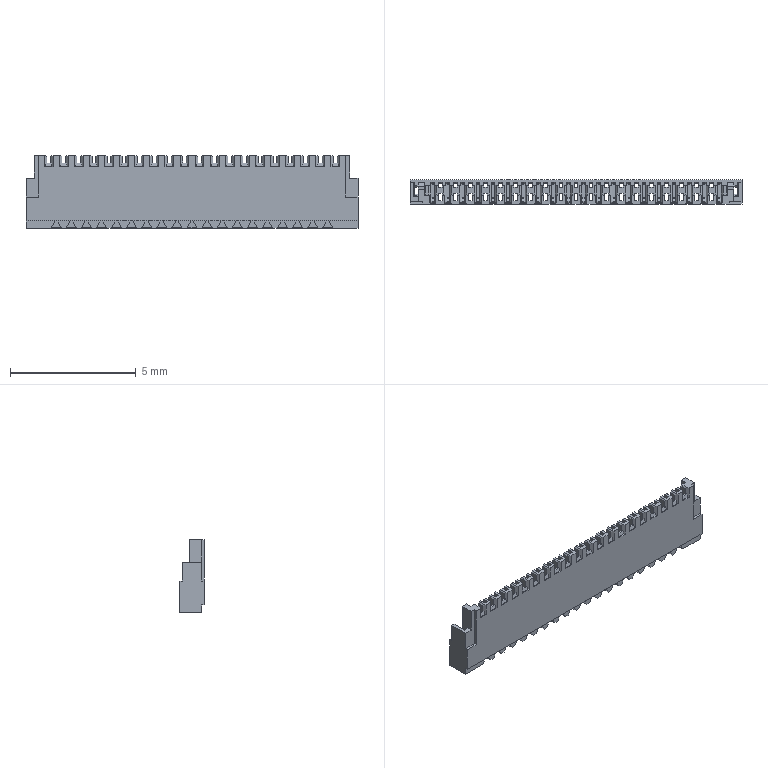Part | Creo | 1 solid | 851 faces | box 13.2 x 0.97 x 2.9 mm | volume 14.533 mm3 | plane 813 | cylinder 38 | commonest cylinder face diameters 0.2 x38